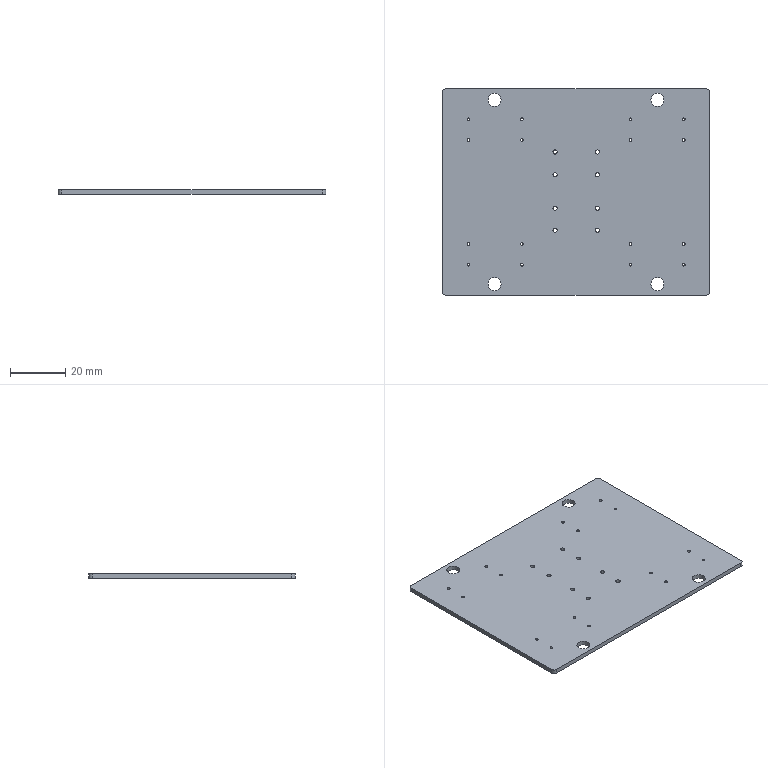Part | STEP file | SOLID | 1 solid | 38 faces | box 96.757 x 74.5 x 1.6 mm | volume 11377 mm3 | cylinder 32 | plane 6 | commonest cylinder face diameters 1 x16 1.5 x8 2.54 x4 4.7 x4